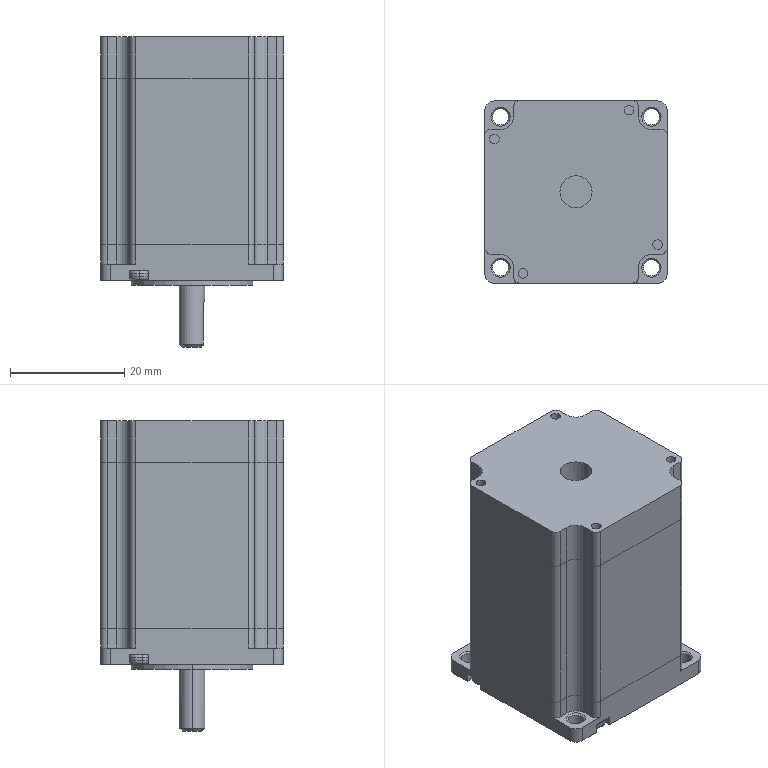Part | SolidWorks | features BaseBody 8, Scale 2 | 8 solids | 273 faces | box 31.92 x 31.92 x 54.32 mm | volume 39661 mm3 | plane 160 | cylinder 83 | torus 20 | cone 10 | commonest cylinder face diameters 2.24 x24 3.36 x19 4.48 x16 1.68 x8 2.8 x8 5.6 x6